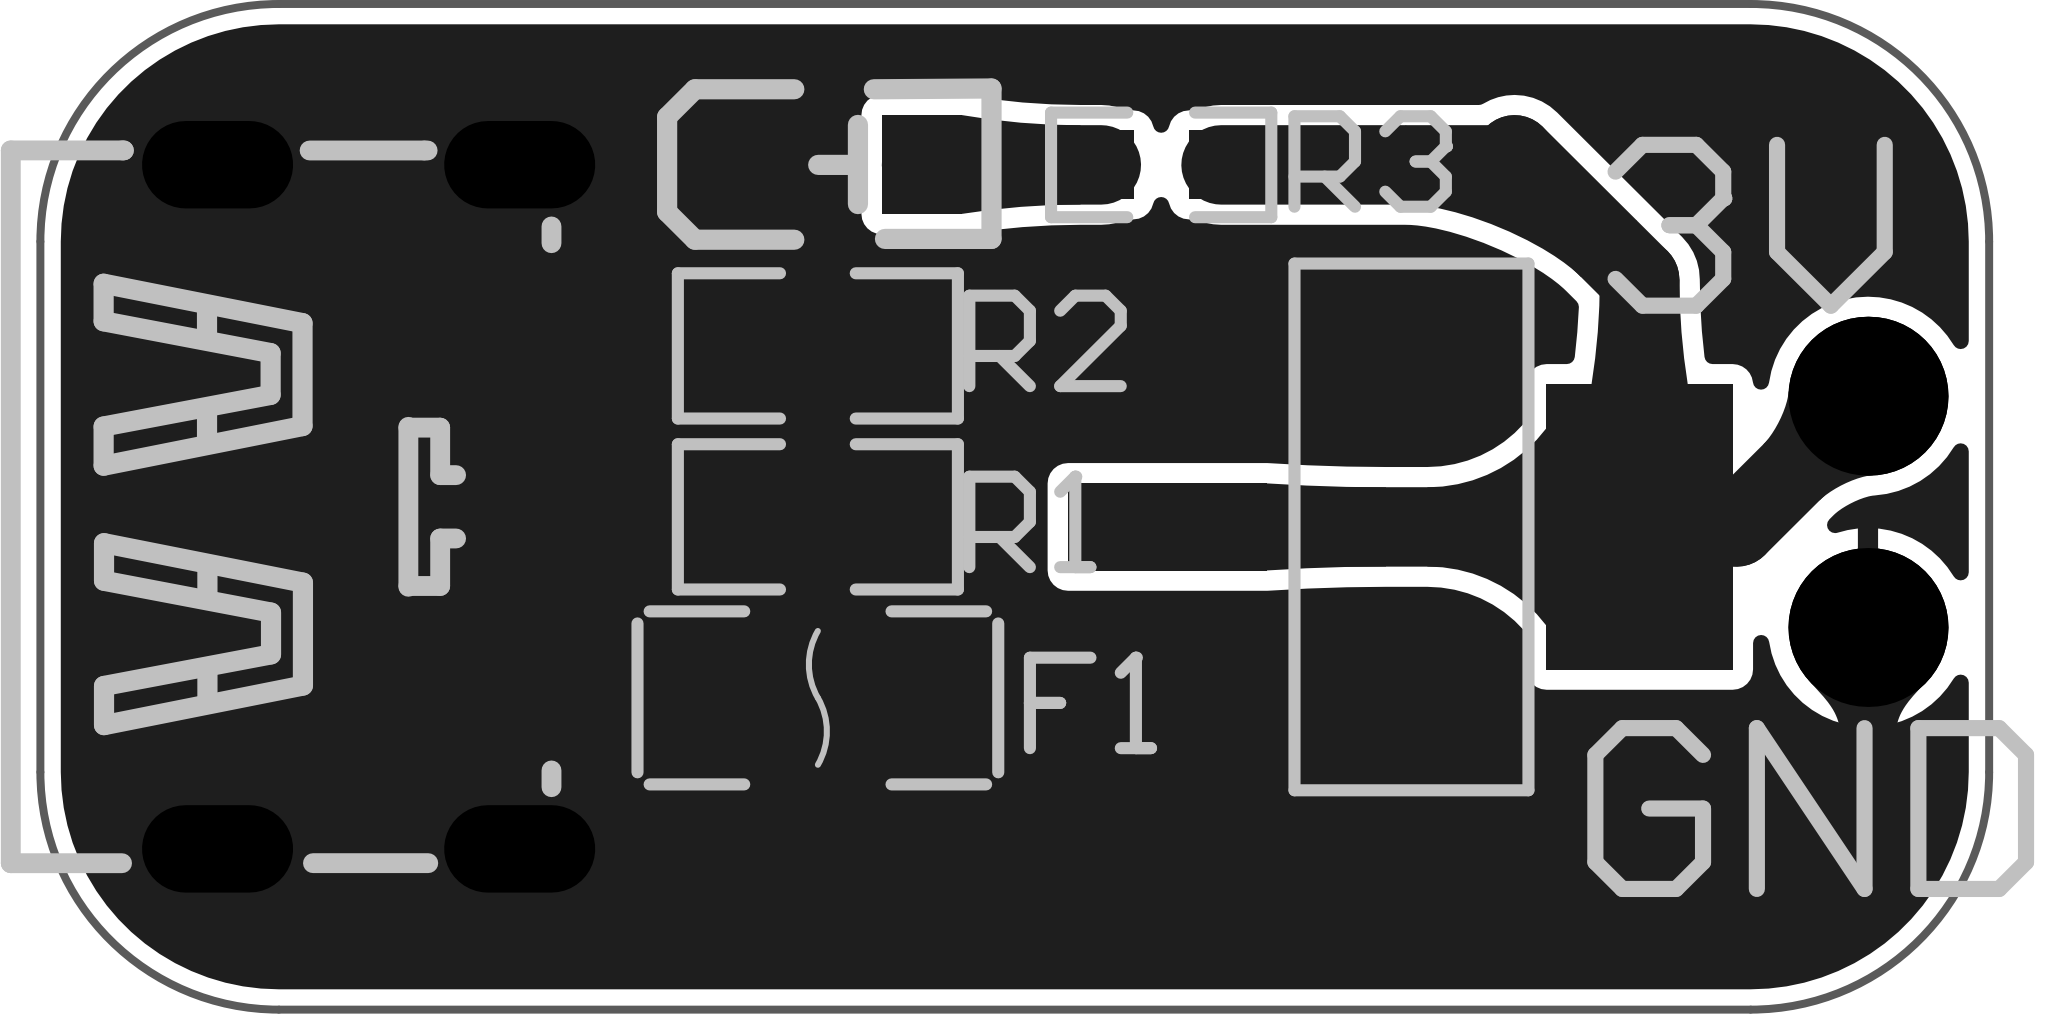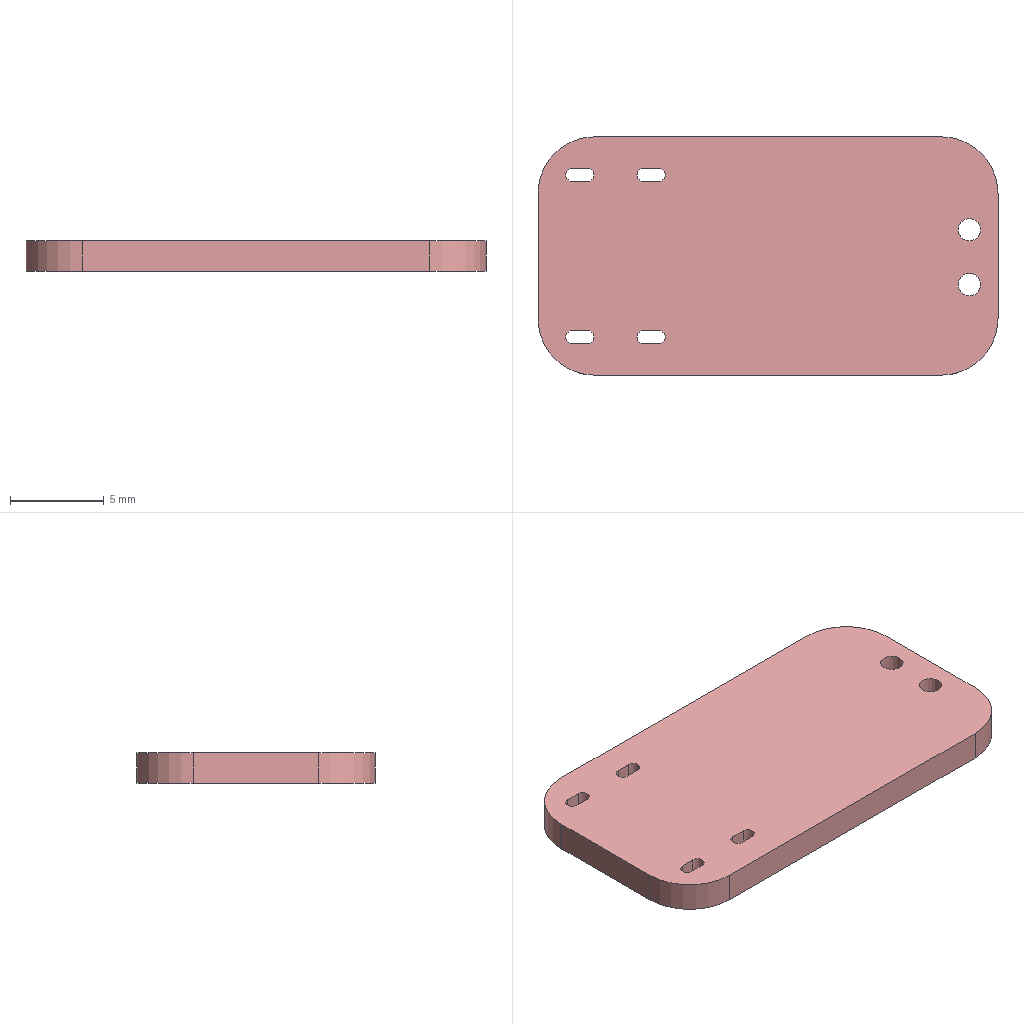Circuit board layout | Altium Designer | box 24.5 x 12.7 x 1.6 mm
Layer stack:
# Altium Designer layer stack of  (unit mm; dielectric type: 0 none, 1 core, 2 prepreg, 3 surface material)
index,name,kind,layer,copper_thickness_mm,dielectric_type,dielectric_thickness_mm,dielectric_material,dielectric_constant
0,Top Paste Mask Layer,other,,,,,,
1,Top Silkscreen Layer,other,,,,,,
2,Top Solder Mask Layer,dielectric,,,3,0.01,,3.3
3,Top Layer,copper,Top Layer,0.035,,,,
4,Dielectric1,dielectric,,,3,1.51,FR4,4.5
5,Bottom Layer,copper,Bottom Layer,0.035,,,,
6,Bottom Solder Mask Layer,dielectric,,,3,0.01,,3.3
7,Bottom Silkscreen Layer,other,,,,,,
8,Bottom Paste Mask Layer,other,,,,,,
# drill layer pairs: low layer,high layer
drill_pair,Top Layer,Bottom Layer
Part placement:
Designator,Comment,Layer,Footprint,Center-X(mm),Center-Y(mm),Rotation
R1,5.1k,TopLayer,R0805,200.914,83.947,0
R2,5.1k,TopLayer,R0805,200.914,86.106,0
USB1,TYPE_C_SMD_6P,TopLayer,TYPE-C-SMD_TYPE-C-6P,195.326,84.074,270
U1,AMS1117-3.3,TopLayer,SOT-223-3_L6.5-W3.4-P2.30-LS7.0-BR,208.28,83.82,180
LED1,,TopLayer,LED_0805,201.118,88.397,0
R3,1K,TopLayer,R0603,205.232,88.392,180
F1,BSMD1206-200-6V,TopLayer,F1206,200.914,81.661,180
Pad and via stacks:
# Altium Designer via and pad stacks of  (unit mm). Each distinct definition once, with the count of objects using it.
# via: kind,start_layer,end_layer,hole_mm,diameter_mm,mode(0 simple;1 top-mid-bottom;2 full stack),diameter_per_layer,count,example_net
# pad: kind,layer,hole_mm,hole_type(0 round;1 square;2 slot),plating,top_size,top_shape(1 round;2 rect;3 octagon;9 rounded rect),mid_size,bottom_size,mode,footprint,size_per_layer,count,example
pad,Multi-Layer,1.2,0,plated,2x2,1,2x2,2x2,0,,,2,1
pad,Multi-Layer,0.7,2,plated,1.1x1.9,1,1.1x1.9,1.1x1.9,0,TYPE-C-SMD_TYPE-C-6P,,4,USB1.7
pad,Top Layer,0,0,plated,1.133x1.377,2,1.133x1.377,1.133x1.377,0,R0805,,4,R1.2
pad,Top Layer,0,0,plated,0.8x1,2,0.8x1,0.8x1,0,TYPE-C-SMD_TYPE-C-6P,,2,USB1.B12
pad,Top Layer,0,0,plated,0.7x1,2,0.7x1,0.7x1,0,TYPE-C-SMD_TYPE-C-6P,,4,USB1.B9
pad,Top Layer,0,0,plated,2.5x1.1,2,2.5x1.1,2.5x1.1,0,SOT-223-3_L6.5-W3.4-P2.30-LS7.0-BR,,3,U1.1
pad,Top Layer,0,0,plated,2.34x3.6,2,2.34x3.6,2.34x3.6,0,SOT-223-3_L6.5-W3.4-P2.30-LS7.0-BR,,1,U1.4
pad,Top Layer,0,0,plated,1x1.25,2,1x1.25,1x1.25,0,LED_0805,,2,LED1.2
pad,Top Layer,0,0,plated,0.8065x0.864,2,0.8065x0.864,0.8065x0.864,0,R0603,,2,R3.2
pad,Top Layer,0,0,plated,1.19x1.728,2,1.19x1.728,1.19x1.728,0,F1206,,2,F1.1
Copper pours:
name,layer,net,type(0 solid;1 hatched;2 none)
Top Layer-GND,Top Layer,GND,0
Top Layer-GND 1,Top Layer,GND,0
Bottom Layer-GND,Bottom Layer,GND,0
Design rules, without the lines most boards share:
# Altium Designer design rules of  (exported by Altium Designer, unit mm)
# columns: name | kind | enabled | priority | scope1 | scope2 | descriptor | typed fields (field=value)
otherClearance | 52 | enabled | 1 | All | All | Hole To Hole Clearance (Gap=11.8mil) (All),(All) | gap=0.2997